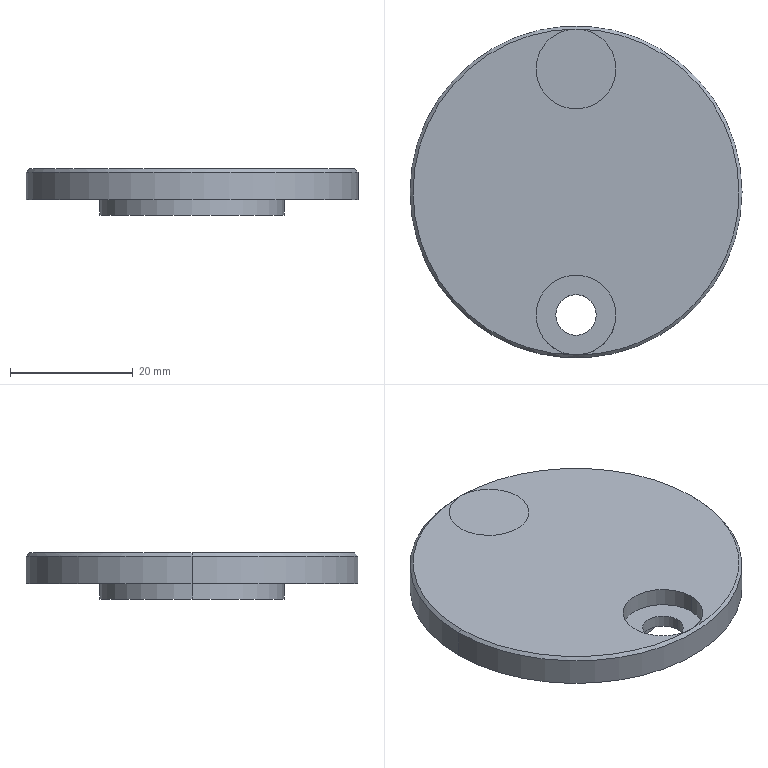Part | SolidWorks | features 3DProfileFeature 1, Chamfer 1, Extrusion 1, HoleWzd 1, ICE 1 | 1 solid | 19 faces | box 54 x 54 x 7.5 mm | volume 12264 mm3 | cylinder 12 | plane 5 | cone 2 | commonest cylinder face diameters 6.6 x4 13 x4 30 x2 54 x2
STEP:
#1=CARTESIAN_POINT('',(26.5,0.,7.5));
#2=VERTEX_POINT('',#1);
#3=CARTESIAN_POINT('',(0.,26.5,7.5));
#4=VERTEX_POINT('',#3);
#5=CARTESIAN_POINT('',(0.,0.,7.5));
#6=DIRECTION('',(0.,0.,1.));
#7=DIRECTION('',(1.,0.,0.));
#8=AXIS2_PLACEMENT_3D('',#5,#6,#7);
#9=CIRCLE('',#8,26.5);
#10=EDGE_CURVE('',#2,#4,#9,.T.);
#11=ORIENTED_EDGE('',*,*,#10,.F.);
#12=CARTESIAN_POINT('',(27.,0.,7.));
#13=VERTEX_POINT('',#12);
#14=CARTESIAN_POINT('',(26.5,0.,7.5));
#15=DIRECTION('',(0.7071,0.,-0.7071));
#16=VECTOR('',#15,1000.);
#17=LINE('',#14,#16);
#18=EDGE_CURVE('',#2,#13,#17,.T.);
#19=ORIENTED_EDGE('',*,*,#18,.T.);
#20=CARTESIAN_POINT('',(-27.,0.,7.));
#21=VERTEX_POINT('',#20);
#22=CARTESIAN_POINT('',(0.,0.,7.));
#23=DIRECTION('',(0.,0.,-1.));
#24=DIRECTION('',(1.,0.,0.));
#25=AXIS2_PLACEMENT_3D('',#22,#23,#24);
#26=CIRCLE('',#25,27.);
#27=EDGE_CURVE('',#21,#13,#26,.T.);
#28=ORIENTED_EDGE('',*,*,#27,.F.);
#29=CARTESIAN_POINT('',(-26.5,0.,7.5));
#30=VERTEX_POINT('',#29);
#31=CARTESIAN_POINT('',(-26.5,0.,7.5));
#32=DIRECTION('',(-0.7071,0.,-0.7071));
#33=VECTOR('',#32,1000.);
#34=LINE('',#31,#33);
#35=EDGE_CURVE('',#30,#21,#34,.T.);
#36=ORIENTED_EDGE('',*,*,#35,.F.);
#37=CARTESIAN_POINT('',(0.,0.,7.5));
#38=DIRECTION('',(0.,0.,1.));
#39=DIRECTION('',(1.,0.,0.));
#40=AXIS2_PLACEMENT_3D('',#37,#38,#39);
#41=CIRCLE('',#40,26.5);
#42=EDGE_CURVE('',#4,#30,#41,.T.);
#43=ORIENTED_EDGE('',*,*,#42,.F.);
#44=EDGE_LOOP('',(#11,#19,#28,#36,#43));
#45=FACE_OUTER_BOUND('',#44,.T.);
#46=CARTESIAN_POINT('',(0.,0.,7.5));
#47=DIRECTION('',(0.,0.,-1.));
#48=DIRECTION('',(-1.,0.,0.));
#49=AXIS2_PLACEMENT_3D('',#46,#47,#48);
#50=CONICAL_SURFACE('',#49,26.5,0.7854);
#51=ADVANCED_FACE('',(#45),#50,.T.);
#52=CARTESIAN_POINT('',(-6.5,20.,4.5));
#53=VERTEX_POINT('',#52);
#54=CARTESIAN_POINT('',(6.5,20.,4.5));
#55=VERTEX_POINT('',#54);
#56=CARTESIAN_POINT('',(0.,20.,4.5));
#57=DIRECTION('',(0.,0.,1.));
#58=DIRECTION('',(1.,0.,0.));
#59=AXIS2_PLACEMENT_3D('',#56,#57,#58);
#60=CIRCLE('',#59,6.5);
#61=EDGE_CURVE('',#53,#55,#60,.T.);
#62=ORIENTED_EDGE('',*,*,#61,.F.);
#63=CARTESIAN_POINT('',(-6.5,20.,7.5));
#64=VERTEX_POINT('',#63);
#65=CARTESIAN_POINT('',(-6.5,20.,7.5));
#66=DIRECTION('',(0.,0.,1.));
#67=VECTOR('',#66,1000.);
#68=LINE('',#65,#67);
#69=EDGE_CURVE('',#53,#64,#68,.T.);
#70=ORIENTED_EDGE('',*,*,#69,.T.);
#71=CARTESIAN_POINT('',(6.5,20.,7.5));
#72=VERTEX_POINT('',#71);
#73=CARTESIAN_POINT('',(0.,20.,7.5));
#74=DIRECTION('',(0.,0.,1.));
#75=DIRECTION('',(1.,0.,0.));
#76=AXIS2_PLACEMENT_3D('',#73,#74,#75);
#77=CIRCLE('',#76,6.5);
#78=EDGE_CURVE('',#64,#72,#77,.T.);
#79=ORIENTED_EDGE('',*,*,#78,.T.);
#80=CARTESIAN_POINT('',(6.5,20.,7.5));
#81=DIRECTION('',(0.,0.,1.));
#82=VECTOR('',#81,1000.);
#83=LINE('',#80,#82);
#84=EDGE_CURVE('',#55,#72,#83,.T.);
#85=ORIENTED_EDGE('',*,*,#84,.F.);
#86=EDGE_LOOP('',(#62,#70,#79,#85));
#87=FACE_OUTER_BOUND('',#86,.T.);
#88=CARTESIAN_POINT('',(0.,20.,7.5));
#89=DIRECTION('',(0.,0.,1.));
#90=DIRECTION('',(1.,0.,0.));
#91=AXIS2_PLACEMENT_3D('',#88,#89,#90);
#92=CYLINDRICAL_SURFACE('',#91,6.5);
#93=ADVANCED_FACE('',(#87),#92,.F.);
#94=CARTESIAN_POINT('',(-3.3,20.,2.5));
#95=VERTEX_POINT('',#94);
#96=CARTESIAN_POINT('',(3.3,20.,2.5));
#97=VERTEX_POINT('',#96);
#98=CARTESIAN_POINT('',(0.,20.,2.5));
#99=DIRECTION('',(0.,0.,1.));
#100=DIRECTION('',(1.,0.,0.));
#101=AXIS2_PLACEMENT_3D('',#98,#99,#100);
#102=CIRCLE('',#101,3.3);
#103=EDGE_CURVE('',#95,#97,#102,.T.);
#104=ORIENTED_EDGE('',*,*,#103,.F.);
#105=CARTESIAN_POINT('',(-3.3,20.,4.5));
#106=VERTEX_POINT('',#105);
#107=CARTESIAN_POINT('',(-3.3,20.,7.5));
#108=DIRECTION('',(0.,0.,1.));
#109=VECTOR('',#108,1000.);
#110=LINE('',#107,#109);
#111=EDGE_CURVE('',#95,#106,#110,.T.);
#112=ORIENTED_EDGE('',*,*,#111,.T.);
#113=CARTESIAN_POINT('',(3.3,20.,4.5));
#114=VERTEX_POINT('',#113);
#115=CARTESIAN_POINT('',(0.,20.,4.5));
#116=DIRECTION('',(0.,0.,1.));
#117=DIRECTION('',(1.,0.,0.));
#118=AXIS2_PLACEMENT_3D('',#115,#116,#117);
#119=CIRCLE('',#118,3.3);
#120=EDGE_CURVE('',#106,#114,#119,.T.);
#121=ORIENTED_EDGE('',*,*,#120,.T.);
#122=CARTESIAN_POINT('',(3.3,20.,7.5));
#123=DIRECTION('',(0.,0.,1.));
#124=VECTOR('',#123,1000.);
#125=LINE('',#122,#124);
#126=EDGE_CURVE('',#97,#114,#125,.T.);
#127=ORIENTED_EDGE('',*,*,#126,.F.);
#128=EDGE_LOOP('',(#104,#112,#121,#127));
#129=FACE_OUTER_BOUND('',#128,.T.);
#130=CARTESIAN_POINT('',(0.,20.,7.5));
#131=DIRECTION('',(0.,0.,1.));
#132=DIRECTION('',(1.,0.,0.));
#133=AXIS2_PLACEMENT_3D('',#130,#131,#132);
#134=CYLINDRICAL_SURFACE('',#133,3.3);
#135=ADVANCED_FACE('',(#129),#134,.F.);
#136=CARTESIAN_POINT('',(-6.5,-20.,4.5));
#137=VERTEX_POINT('',#136);
#138=CARTESIAN_POINT('',(6.5,-20.,4.5));
#139=VERTEX_POINT('',#138);
#140=CARTESIAN_POINT('',(0.,-20.,4.5));
#141=DIRECTION('',(0.,0.,1.));
#142=DIRECTION('',(1.,0.,0.));
#143=AXIS2_PLACEMENT_3D('',#140,#141,#142);
#144=CIRCLE('',#143,6.5);
#145=EDGE_CURVE('',#137,#139,#144,.T.);
#146=ORIENTED_EDGE('',*,*,#145,.F.);
#147=CARTESIAN_POINT('',(-6.5,-20.,7.5));
#148=VERTEX_POINT('',#147);
#149=CARTESIAN_POINT('',(-6.5,-20.,7.5));
#150=DIRECTION('',(0.,0.,1.));
#151=VECTOR('',#150,1000.);
#152=LINE('',#149,#151);
#153=EDGE_CURVE('',#137,#148,#152,.T.);
#154=ORIENTED_EDGE('',*,*,#153,.T.);
#155=CARTESIAN_POINT('',(0.,-26.5,7.5));
#156=VERTEX_POINT('',#155);
#157=CARTESIAN_POINT('',(0.,-20.,7.5));
#158=DIRECTION('',(0.,0.,1.));
#159=DIRECTION('',(1.,0.,0.));
#160=AXIS2_PLACEMENT_3D('',#157,#158,#159);
#161=CIRCLE('',#160,6.5);
#162=EDGE_CURVE('',#148,#156,#161,.T.);
#163=ORIENTED_EDGE('',*,*,#162,.T.);
#164=CARTESIAN_POINT('',(6.5,-20.,7.5));
#165=VERTEX_POINT('',#164);
#166=CARTESIAN_POINT('',(0.,-20.,7.5));
#167=DIRECTION('',(0.,0.,1.));
#168=DIRECTION('',(1.,0.,0.));
#169=AXIS2_PLACEMENT_3D('',#166,#167,#168);
#170=CIRCLE('',#169,6.5);
#171=EDGE_CURVE('',#156,#165,#170,.T.);
#172=ORIENTED_EDGE('',*,*,#171,.T.);
#173=CARTESIAN_POINT('',(6.5,-20.,7.5));
#174=DIRECTION('',(0.,0.,1.));
#175=VECTOR('',#174,1000.);
#176=LINE('',#173,#175);
#177=EDGE_CURVE('',#139,#165,#176,.T.);
#178=ORIENTED_EDGE('',*,*,#177,.F.);
#179=EDGE_LOOP('',(#146,#154,#163,#172,#178));
#180=FACE_OUTER_BOUND('',#179,.T.);
#181=CARTESIAN_POINT('',(0.,-20.,7.5));
#182=DIRECTION('',(0.,0.,1.));
#183=DIRECTION('',(1.,0.,0.));
#184=AXIS2_PLACEMENT_3D('',#181,#182,#183);
#185=CYLINDRICAL_SURFACE('',#184,6.5);
#186=ADVANCED_FACE('',(#180),#185,.F.);
#187=CARTESIAN_POINT('',(-3.3,-20.,2.5));
#188=VERTEX_POINT('',#187);
#189=CARTESIAN_POINT('',(3.3,-20.,2.5));
#190=VERTEX_POINT('',#189);
#191=CARTESIAN_POINT('',(0.,-20.,2.5));
#192=DIRECTION('',(0.,0.,1.));
#193=DIRECTION('',(1.,0.,0.));
#194=AXIS2_PLACEMENT_3D('',#191,#192,#193);
#195=CIRCLE('',#194,3.3);
#196=EDGE_CURVE('',#188,#190,#195,.T.);
#197=ORIENTED_EDGE('',*,*,#196,.F.);
#198=CARTESIAN_POINT('',(-3.3,-20.,4.5));
#199=VERTEX_POINT('',#198);
#200=CARTESIAN_POINT('',(-3.3,-20.,7.5));
#201=DIRECTION('',(0.,0.,1.));
#202=VECTOR('',#201,1000.);
#203=LINE('',#200,#202);
#204=EDGE_CURVE('',#188,#199,#203,.T.);
#205=ORIENTED_EDGE('',*,*,#204,.T.);
#206=CARTESIAN_POINT('',(3.3,-20.,4.5));
#207=VERTEX_POINT('',#206);
#208=CARTESIAN_POINT('',(0.,-20.,4.5));
#209=DIRECTION('',(0.,0.,1.));
#210=DIRECTION('',(1.,0.,0.));
#211=AXIS2_PLACEMENT_3D('',#208,#209,#210);
#212=CIRCLE('',#211,3.3);
#213=EDGE_CURVE('',#199,#207,#212,.T.);
#214=ORIENTED_EDGE('',*,*,#213,.T.);
#215=CARTESIAN_POINT('',(3.3,-20.,7.5));
#216=DIRECTION('',(0.,0.,1.));
#217=VECTOR('',#216,1000.);
#218=LINE('',#215,#217);
#219=EDGE_CURVE('',#190,#207,#218,.T.);
#220=ORIENTED_EDGE('',*,*,#219,.F.);
#221=EDGE_LOOP('',(#197,#205,#214,#220));
#222=FACE_OUTER_BOUND('',#221,.T.);
#223=CARTESIAN_POINT('',(0.,-20.,7.5));
#224=DIRECTION('',(0.,0.,1.));
#225=DIRECTION('',(1.,0.,0.));
#226=AXIS2_PLACEMENT_3D('',#223,#224,#225);
#227=CYLINDRICAL_SURFACE('',#226,3.3);
#228=ADVANCED_FACE('',(#222),#227,.F.);
#229=ORIENTED_EDGE('',*,*,#27,.T.);
#230=CARTESIAN_POINT('',(27.,0.,2.5));
#231=VERTEX_POINT('',#230);
#232=CARTESIAN_POINT('',(27.,0.,7.5));
#233=DIRECTION('',(0.,0.,-1.));
#234=VECTOR('',#233,1000.);
#235=LINE('',#232,#234);
#236=EDGE_CURVE('',#13,#231,#235,.T.);
#237=ORIENTED_EDGE('',*,*,#236,.T.);
#238=CARTESIAN_POINT('',(-27.,0.,2.5));
#239=VERTEX_POINT('',#238);
#240=CARTESIAN_POINT('',(0.,0.,2.5));
#241=DIRECTION('',(0.,0.,1.));
#242=DIRECTION('',(1.,0.,0.));
#243=AXIS2_PLACEMENT_3D('',#240,#241,#242);
#244=CIRCLE('',#243,27.);
#245=EDGE_CURVE('',#231,#239,#244,.T.);
#246=ORIENTED_EDGE('',*,*,#245,.T.);
#247=CARTESIAN_POINT('',(-27.,0.,7.5));
#248=DIRECTION('',(0.,0.,-1.));
#249=VECTOR('',#248,1000.);
#250=LINE('',#247,#249);
#251=EDGE_CURVE('',#21,#239,#250,.T.);
#252=ORIENTED_EDGE('',*,*,#251,.F.);
#253=EDGE_LOOP('',(#229,#237,#246,#252));
#254=FACE_OUTER_BOUND('',#253,.T.);
#255=CARTESIAN_POINT('',(0.,0.,7.5));
#256=DIRECTION('',(0.,0.,-1.));
#257=DIRECTION('',(-1.,0.,0.));
#258=AXIS2_PLACEMENT_3D('',#255,#256,#257);
#259=CYLINDRICAL_SURFACE('',#258,27.);
#260=ADVANCED_FACE('',(#254),#259,.T.);
#261=CARTESIAN_POINT('',(15.,0.,2.5));
#262=VERTEX_POINT('',#261);
#263=CARTESIAN_POINT('',(-15.,0.,2.5));
#264=VERTEX_POINT('',#263);
#265=CARTESIAN_POINT('',(0.,0.,2.5));
#266=DIRECTION('',(0.,0.,1.));
#267=DIRECTION('',(1.,0.,0.));
#268=AXIS2_PLACEMENT_3D('',#265,#266,#267);
#269=CIRCLE('',#268,15.);
#270=EDGE_CURVE('',#262,#264,#269,.T.);
#271=ORIENTED_EDGE('',*,*,#270,.F.);
#272=CARTESIAN_POINT('',(15.,0.,0.));
#273=VERTEX_POINT('',#272);
#274=CARTESIAN_POINT('',(15.,0.,2.5));
#275=DIRECTION('',(0.,0.,-1.));
#276=VECTOR('',#275,1000.);
#277=LINE('',#274,#276);
#278=EDGE_CURVE('',#262,#273,#277,.T.);
#279=ORIENTED_EDGE('',*,*,#278,.T.);
#280=CARTESIAN_POINT('',(-15.,0.,0.));
#281=VERTEX_POINT('',#280);
#282=CARTESIAN_POINT('',(0.,0.,0.));
#283=DIRECTION('',(0.,0.,1.));
#284=DIRECTION('',(1.,0.,0.));
#285=AXIS2_PLACEMENT_3D('',#282,#283,#284);
#286=CIRCLE('',#285,15.);
#287=EDGE_CURVE('',#273,#281,#286,.T.);
#288=ORIENTED_EDGE('',*,*,#287,.T.);
#289=CARTESIAN_POINT('',(-15.,0.,2.5));
#290=DIRECTION('',(0.,0.,-1.));
#291=VECTOR('',#290,1000.);
#292=LINE('',#289,#291);
#293=EDGE_CURVE('',#264,#281,#292,.T.);
#294=ORIENTED_EDGE('',*,*,#293,.F.);
#295=EDGE_LOOP('',(#271,#279,#288,#294));
#296=FACE_OUTER_BOUND('',#295,.T.);
#297=CARTESIAN_POINT('',(0.,0.,2.5));
#298=DIRECTION('',(0.,0.,-1.));
#299=DIRECTION('',(-1.,0.,0.));
#300=AXIS2_PLACEMENT_3D('',#297,#298,#299);
#301=CYLINDRICAL_SURFACE('',#300,15.);
#302=ADVANCED_FACE('',(#296),#301,.T.);
#303=ORIENTED_EDGE('',*,*,#278,.F.);
#304=CARTESIAN_POINT('',(0.,0.,2.5));
#305=DIRECTION('',(0.,0.,1.));
#306=DIRECTION('',(1.,0.,0.));
#307=AXIS2_PLACEMENT_3D('',#304,#305,#306);
#308=CIRCLE('',#307,15.);
#309=EDGE_CURVE('',#264,#262,#308,.T.);
#310=ORIENTED_EDGE('',*,*,#309,.F.);
#311=ORIENTED_EDGE('',*,*,#293,.T.);
#312=CARTESIAN_POINT('',(0.,0.,0.));
#313=DIRECTION('',(0.,0.,1.));
#314=DIRECTION('',(1.,0.,0.));
#315=AXIS2_PLACEMENT_3D('',#312,#313,#314);
#316=CIRCLE('',#315,15.);
#317=EDGE_CURVE('',#281,#273,#316,.T.);
#318=ORIENTED_EDGE('',*,*,#317,.T.);
#319=EDGE_LOOP('',(#303,#310,#311,#318));
#320=FACE_OUTER_BOUND('',#319,.T.);
#321=CARTESIAN_POINT('',(0.,0.,2.5));
#322=DIRECTION('',(0.,0.,-1.));
#323=DIRECTION('',(-1.,0.,0.));
#324=AXIS2_PLACEMENT_3D('',#321,#322,#323);
#325=CYLINDRICAL_SURFACE('',#324,15.);
#326=ADVANCED_FACE('',(#320),#325,.T.);
#327=ORIENTED_EDGE('',*,*,#317,.F.);
#328=ORIENTED_EDGE('',*,*,#287,.F.);
#329=EDGE_LOOP('',(#327,#328));
#330=FACE_OUTER_BOUND('',#329,.T.);
#331=CARTESIAN_POINT('',(0.,0.,0.));
#332=DIRECTION('',(0.,0.,1.));
#333=DIRECTION('',(1.,0.,0.));
#334=AXIS2_PLACEMENT_3D('',#331,#332,#333);
#335=PLANE('',#334);
#336=ADVANCED_FACE('',(#330),#335,.F.);
#337=ORIENTED_EDGE('',*,*,#236,.F.);
#338=CARTESIAN_POINT('',(0.,0.,7.));
#339=DIRECTION('',(0.,0.,-1.));
#340=DIRECTION('',(1.,0.,0.));
#341=AXIS2_PLACEMENT_3D('',#338,#339,#340);
#342=CIRCLE('',#341,27.);
#343=EDGE_CURVE('',#13,#21,#342,.T.);
#344=ORIENTED_EDGE('',*,*,#343,.T.);
#345=ORIENTED_EDGE('',*,*,#251,.T.);
#346=CARTESIAN_POINT('',(0.,0.,2.5));
#347=DIRECTION('',(0.,0.,1.));
#348=DIRECTION('',(1.,0.,0.));
#349=AXIS2_PLACEMENT_3D('',#346,#347,#348);
#350=CIRCLE('',#349,27.);
#351=EDGE_CURVE('',#239,#231,#350,.T.);
#352=ORIENTED_EDGE('',*,*,#351,.T.);
#353=EDGE_LOOP('',(#337,#344,#345,#352));
#354=FACE_OUTER_BOUND('',#353,.T.);
#355=CARTESIAN_POINT('',(0.,0.,7.5));
#356=DIRECTION('',(0.,0.,-1.));
#357=DIRECTION('',(-1.,0.,0.));
#358=AXIS2_PLACEMENT_3D('',#355,#356,#357);
#359=CYLINDRICAL_SURFACE('',#358,27.);
#360=ADVANCED_FACE('',(#354),#359,.T.);
#361=CARTESIAN_POINT('',(0.,20.,7.5));
#362=DIRECTION('',(0.,0.,1.));
#363=DIRECTION('',(1.,0.,0.));
#364=AXIS2_PLACEMENT_3D('',#361,#362,#363);
#365=CIRCLE('',#364,6.5);
#366=EDGE_CURVE('',#4,#64,#365,.T.);
#367=ORIENTED_EDGE('',*,*,#366,.F.);
#368=ORIENTED_EDGE('',*,*,#42,.T.);
#369=CARTESIAN_POINT('',(0.,0.,7.5));
#370=DIRECTION('',(0.,0.,1.));
#371=DIRECTION('',(1.,0.,0.));
#372=AXIS2_PLACEMENT_3D('',#369,#370,#371);
#373=CIRCLE('',#372,26.5);
#374=EDGE_CURVE('',#30,#156,#373,.T.);
#375=ORIENTED_EDGE('',*,*,#374,.T.);
#376=ORIENTED_EDGE('',*,*,#162,.F.);
#377=CARTESIAN_POINT('',(0.,-20.,7.5));
#378=DIRECTION('',(0.,0.,1.));
#379=DIRECTION('',(1.,0.,0.));
#380=AXIS2_PLACEMENT_3D('',#377,#378,#379);
#381=CIRCLE('',#380,6.5);
#382=EDGE_CURVE('',#165,#148,#381,.T.);
#383=ORIENTED_EDGE('',*,*,#382,.F.);
#384=ORIENTED_EDGE('',*,*,#171,.F.);
#385=CARTESIAN_POINT('',(0.,0.,7.5));
#386=DIRECTION('',(0.,0.,1.));
#387=DIRECTION('',(1.,0.,0.));
#388=AXIS2_PLACEMENT_3D('',#385,#386,#387);
#389=CIRCLE('',#388,26.5);
#390=EDGE_CURVE('',#156,#2,#389,.T.);
#391=ORIENTED_EDGE('',*,*,#390,.T.);
#392=ORIENTED_EDGE('',*,*,#10,.T.);
#393=CARTESIAN_POINT('',(0.,20.,7.5));
#394=DIRECTION('',(0.,0.,1.));
#395=DIRECTION('',(1.,0.,0.));
#396=AXIS2_PLACEMENT_3D('',#393,#394,#395);
#397=CIRCLE('',#396,6.5);
#398=EDGE_CURVE('',#72,#4,#397,.T.);
#399=ORIENTED_EDGE('',*,*,#398,.F.);
#400=ORIENTED_EDGE('',*,*,#78,.F.);
#401=EDGE_LOOP('',(#367,#368,#375,#376,#383,#384,#391,#392,#399,#400));
#402=FACE_OUTER_BOUND('',#401,.T.);
#403=CARTESIAN_POINT('',(0.,0.,7.5));
#404=DIRECTION('',(0.,0.,1.));
#405=DIRECTION('',(1.,0.,0.));
#406=AXIS2_PLACEMENT_3D('',#403,#404,#405);
#407=PLANE('',#406);
#408=ADVANCED_FACE('',(#402),#407,.T.);
#409=CARTESIAN_POINT('',(0.,20.,2.5));
#410=DIRECTION('',(0.,0.,1.));
#411=DIRECTION('',(1.,0.,0.));
#412=AXIS2_PLACEMENT_3D('',#409,#410,#411);
#413=CIRCLE('',#412,3.3);
#414=EDGE_CURVE('',#97,#95,#413,.T.);
#415=ORIENTED_EDGE('',*,*,#414,.T.);
#416=ORIENTED_EDGE('',*,*,#103,.T.);
#417=EDGE_LOOP('',(#415,#416));
#418=FACE_BOUND('',#417,.T.);
#419=CARTESIAN_POINT('',(0.,-20.,2.5));
#420=DIRECTION('',(0.,0.,1.));
#421=DIRECTION('',(1.,0.,0.));
#422=AXIS2_PLACEMENT_3D('',#419,#420,#421);
#423=CIRCLE('',#422,3.3);
#424=EDGE_CURVE('',#190,#188,#423,.T.);
#425=ORIENTED_EDGE('',*,*,#424,.T.);
#426=ORIENTED_EDGE('',*,*,#196,.T.);
#427=EDGE_LOOP('',(#425,#426));
#428=FACE_BOUND('',#427,.T.);
#429=ORIENTED_EDGE('',*,*,#309,.T.);
#430=ORIENTED_EDGE('',*,*,#270,.T.);
#431=EDGE_LOOP('',(#429,#430));
#432=FACE_BOUND('',#431,.T.);
#433=ORIENTED_EDGE('',*,*,#351,.F.);
#434=ORIENTED_EDGE('',*,*,#245,.F.);
#435=EDGE_LOOP('',(#433,#434));
#436=FACE_OUTER_BOUND('',#435,.T.);
#437=CARTESIAN_POINT('',(0.,0.,2.5));
#438=DIRECTION('',(0.,0.,1.));
#439=DIRECTION('',(1.,0.,0.));
#440=AXIS2_PLACEMENT_3D('',#437,#438,#439);
#441=PLANE('',#440);
#442=ADVANCED_FACE('',(#418,#428,#432,#436),#441,.F.);
#443=ORIENTED_EDGE('',*,*,#204,.F.);
#444=ORIENTED_EDGE('',*,*,#424,.F.);
#445=ORIENTED_EDGE('',*,*,#219,.T.);
#446=CARTESIAN_POINT('',(0.,-20.,4.5));
#447=DIRECTION('',(0.,0.,1.));
#448=DIRECTION('',(1.,0.,0.));
#449=AXIS2_PLACEMENT_3D('',#446,#447,#448);
#450=CIRCLE('',#449,3.3);
#451=EDGE_CURVE('',#207,#199,#450,.T.);
#452=ORIENTED_EDGE('',*,*,#451,.T.);
#453=EDGE_LOOP('',(#443,#444,#445,#452));
#454=FACE_OUTER_BOUND('',#453,.T.);
#455=CARTESIAN_POINT('',(0.,-20.,7.5));
#456=DIRECTION('',(0.,0.,1.));
#457=DIRECTION('',(1.,0.,0.));
#458=AXIS2_PLACEMENT_3D('',#455,#456,#457);
#459=CYLINDRICAL_SURFACE('',#458,3.3);
#460=ADVANCED_FACE('',(#454),#459,.F.);
#461=ORIENTED_EDGE('',*,*,#451,.F.);
#462=ORIENTED_EDGE('',*,*,#213,.F.);
#463=EDGE_LOOP('',(#461,#462));
#464=FACE_BOUND('',#463,.T.);
#465=CARTESIAN_POINT('',(0.,-20.,4.5));
#466=DIRECTION('',(0.,0.,1.));
#467=DIRECTION('',(1.,0.,0.));
#468=AXIS2_PLACEMENT_3D('',#465,#466,#467);
#469=CIRCLE('',#468,6.5);
#470=EDGE_CURVE('',#139,#137,#469,.T.);
#471=ORIENTED_EDGE('',*,*,#470,.T.);
#472=ORIENTED_EDGE('',*,*,#145,.T.);
#473=EDGE_LOOP('',(#471,#472));
#474=FACE_OUTER_BOUND('',#473,.T.);
#475=CARTESIAN_POINT('',(3.3,-20.,4.5));
#476=DIRECTION('',(0.,0.,-1.));
#477=DIRECTION('',(-1.,0.,0.));
#478=AXIS2_PLACEMENT_3D('',#475,#476,#477);
#479=PLANE('',#478);
#480=ADVANCED_FACE('',(#464,#474),#479,.F.);
#481=ORIENTED_EDGE('',*,*,#153,.F.);
#482=ORIENTED_EDGE('',*,*,#470,.F.);
#483=ORIENTED_EDGE('',*,*,#177,.T.);
#484=ORIENTED_EDGE('',*,*,#382,.T.);
#485=EDGE_LOOP('',(#481,#482,#483,#484));
#486=FACE_OUTER_BOUND('',#485,.T.);
#487=CARTESIAN_POINT('',(0.,-20.,7.5));
#488=DIRECTION('',(0.,0.,1.));
#489=DIRECTION('',(1.,0.,0.));
#490=AXIS2_PLACEMENT_3D('',#487,#488,#489);
#491=CYLINDRICAL_SURFACE('',#490,6.5);
#492=ADVANCED_FACE('',(#486),#491,.F.);
#493=ORIENTED_EDGE('',*,*,#111,.F.);
#494=ORIENTED_EDGE('',*,*,#414,.F.);
#495=ORIENTED_EDGE('',*,*,#126,.T.);
#496=CARTESIAN_POINT('',(0.,20.,4.5));
#497=DIRECTION('',(0.,0.,1.));
#498=DIRECTION('',(1.,0.,0.));
#499=AXIS2_PLACEMENT_3D('',#496,#497,#498);
#500=CIRCLE('',#499,3.3);
#501=EDGE_CURVE('',#114,#106,#500,.T.);
#502=ORIENTED_EDGE('',*,*,#501,.T.);
#503=EDGE_LOOP('',(#493,#494,#495,#502));
#504=FACE_OUTER_BOUND('',#503,.T.);
#505=CARTESIAN_POINT('',(0.,20.,7.5));
#506=DIRECTION('',(0.,0.,1.));
#507=DIRECTION('',(1.,0.,0.));
#508=AXIS2_PLACEMENT_3D('',#505,#506,#507);
#509=CYLINDRICAL_SURFACE('',#508,3.3);
#510=ADVANCED_FACE('',(#504),#509,.F.);
#511=ORIENTED_EDGE('',*,*,#501,.F.);
#512=ORIENTED_EDGE('',*,*,#120,.F.);
#513=EDGE_LOOP('',(#511,#512));
#514=FACE_BOUND('',#513,.T.);
#515=CARTESIAN_POINT('',(0.,20.,4.5));
#516=DIRECTION('',(0.,0.,1.));
#517=DIRECTION('',(1.,0.,0.));
#518=AXIS2_PLACEMENT_3D('',#515,#516,#517);
#519=CIRCLE('',#518,6.5);
#520=EDGE_CURVE('',#55,#53,#519,.T.);
#521=ORIENTED_EDGE('',*,*,#520,.T.);
#522=ORIENTED_EDGE('',*,*,#61,.T.);
#523=EDGE_LOOP('',(#521,#522));
#524=FACE_OUTER_BOUND('',#523,.T.);
#525=CARTESIAN_POINT('',(3.3,20.,4.5));
#526=DIRECTION('',(0.,0.,-1.));
#527=DIRECTION('',(-1.,0.,0.));
#528=AXIS2_PLACEMENT_3D('',#525,#526,#527);
#529=PLANE('',#528);
#530=ADVANCED_FACE('',(#514,#524),#529,.F.);
#531=ORIENTED_EDGE('',*,*,#69,.F.);
#532=ORIENTED_EDGE('',*,*,#520,.F.);
#533=ORIENTED_EDGE('',*,*,#84,.T.);
#534=ORIENTED_EDGE('',*,*,#398,.T.);
#535=ORIENTED_EDGE('',*,*,#366,.T.);
#536=EDGE_LOOP('',(#531,#532,#533,#534,#535));
#537=FACE_OUTER_BOUND('',#536,.T.);
#538=CARTESIAN_POINT('',(0.,20.,7.5));
#539=DIRECTION('',(0.,0.,1.));
#540=DIRECTION('',(1.,0.,0.));
#541=AXIS2_PLACEMENT_3D('',#538,#539,#540);
#542=CYLINDRICAL_SURFACE('',#541,6.5);
#543=ADVANCED_FACE('',(#537),#542,.F.);
#544=ORIENTED_EDGE('',*,*,#18,.F.);
#545=ORIENTED_EDGE('',*,*,#390,.F.);
#546=ORIENTED_EDGE('',*,*,#374,.F.);
#547=ORIENTED_EDGE('',*,*,#35,.T.);
#548=ORIENTED_EDGE('',*,*,#343,.F.);
#549=EDGE_LOOP('',(#544,#545,#546,#547,#548));
#550=FACE_OUTER_BOUND('',#549,.T.);
#551=CARTESIAN_POINT('',(0.,0.,7.5));
#552=DIRECTION('',(0.,0.,-1.));
#553=DIRECTION('',(-1.,0.,0.));
#554=AXIS2_PLACEMENT_3D('',#551,#552,#553);
#555=CONICAL_SURFACE('',#554,26.5,0.7854);
#556=ADVANCED_FACE('',(#550),#555,.T.);
#557=CLOSED_SHELL('',(#51,#93,#135,#186,#228,#260,#302,#326,#336,#360,#408,#442,#460,#480,#492,#510,#530,#543,#556));
#558=MANIFOLD_SOLID_BREP('',#557);
#559=CARTESIAN_POINT('',(0.,0.,0.));
#560=DIRECTION('',(0.,0.,1.));
#561=DIRECTION('',(1.,0.,0.));
#562=AXIS2_PLACEMENT_3D('',#559,#560,#561);
#563=(LENGTH_UNIT()NAMED_UNIT(*)SI_UNIT(.MILLI.,.METRE.));
#564=UNCERTAINTY_MEASURE_WITH_UNIT(LENGTH_MEASURE(0.00001),#563,'','');
#565=(NAMED_UNIT(*)PLANE_ANGLE_UNIT()SI_UNIT($,.RADIAN.));
#566=(NAMED_UNIT(*)SI_UNIT($,.STERADIAN.)SOLID_ANGLE_UNIT());
#567=(GEOMETRIC_REPRESENTATION_CONTEXT(3)GLOBAL_UNCERTAINTY_ASSIGNED_CONTEXT((#564))GLOBAL_UNIT_ASSIGNED_CONTEXT((#563,#565,#566))REPRESENTATION_CONTEXT('',''));
#568=ADVANCED_BREP_SHAPE_REPRESENTATION('',(#558,#562),#567);